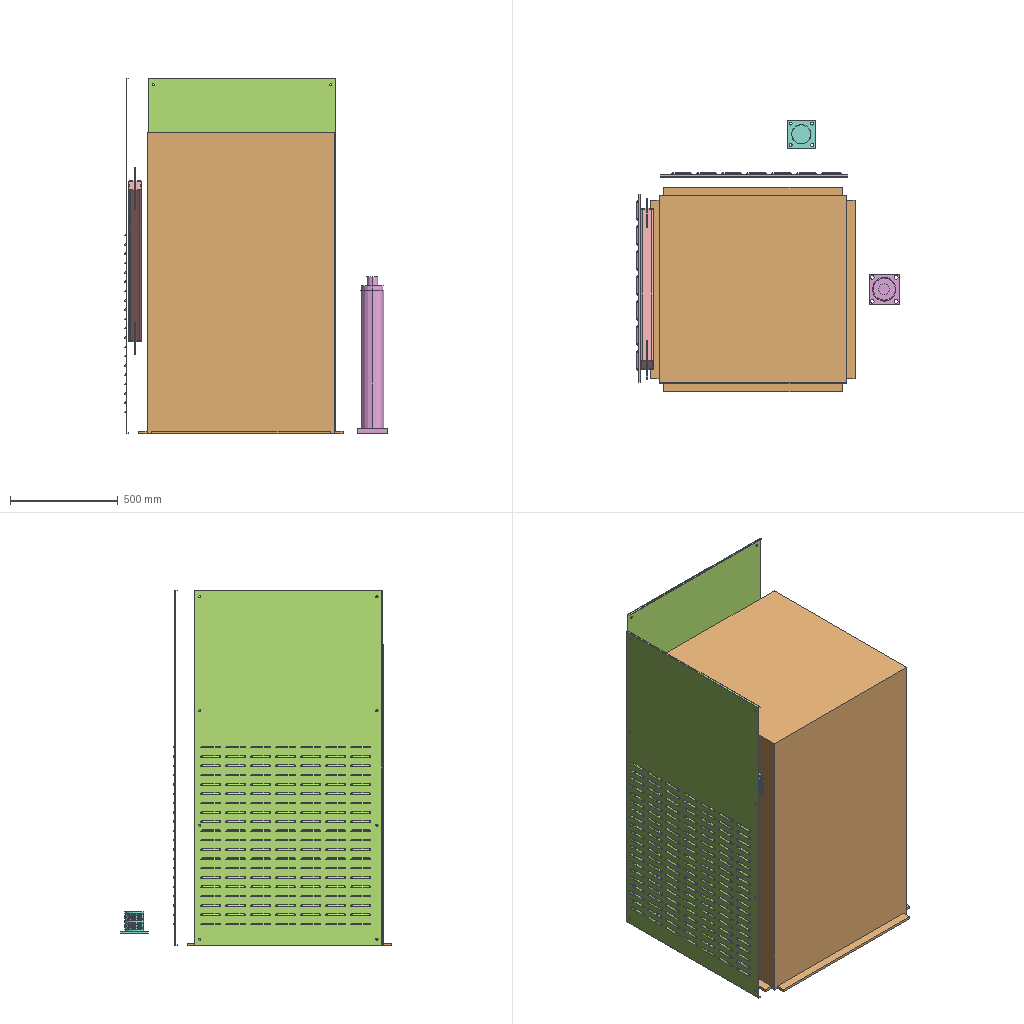Assembly | SolidWorks | 10 different items | 12 placed | box 1219 x 1260 x 1650 mm
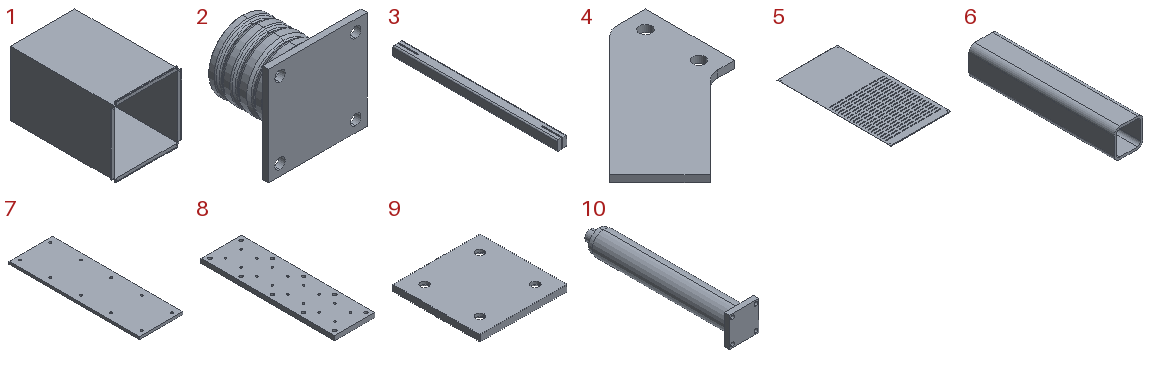Parts list (item | quantity | size | volume | features):
1 | x1 | 950 x 1400 x 950 mm | 61176455 mm3 | features CirPattern 1, Extrusion 1, ICE 1, RefAxis 1, Shell 1
2 | x1 | 130 x 100 x 130 mm | 689791 mm3 | features Chamfer 1, Extrusion 1, Fillet 1, ICE 1, RevCut 1
3 | x1 | 60 x 998 x 60 mm | 853297 mm3 | features ICE 3, Extrusion 1
4 | x2 | 181.644 x 197.856 x 8 mm | 132691 mm3 | features Extrusion 1
5 | x2 | 870 x 1650 x 17.75 mm | 2197633 mm3 | features ICE 5, Fillet 3, LPattern 2, Shell 2, CombineBodies 1, Extrusion 1
6 | x1 | 50 x 250 x 50 mm | 170265 mm3 | features Extrusion 1
7 | x1 | 100 x 300 x 6 mm | 178822 mm3 | features LPattern 2, Extrusion 1, HoleWzd 1
8 | x1 | 90 x 300 x 10 mm | 263935 mm3 | features LPattern 3, HoleWzd 2, Extrusion 1
9 | x1 | 55 x 55 x 4 mm | 11573 mm3 | features Chamfer 1, Extrusion 1, HoleWzd 1
10 | x1 | 140 x 729 x 140 mm | 6809578 mm3 | features ICE 1, Revolution 1
Mates (type | each side: item.copy, entity, surface, feature):
Coincident | 1.1 plane | assembly plane | 2 times
Parallel | 3.1 face plane Boss-Extrude1 | 4.1 face plane Boss-Extrude1
Coincident | 3.1 face plane Cut-Extrude1 | 4.1 face plane Boss-Extrude1
DistanceDim | 3.1 face plane Boss-Extrude1 | 4.1 edge
DistanceDim | 3.1 edge | 4.1 face plane Boss-Extrude1
Parallel | 3.1 face plane Cut-Extrude1 | 4.2 face plane Boss-Extrude1
Parallel | 3.1 face plane Boss-Extrude1 | 4.2 face plane Boss-Extrude1
DistanceDim | 3.1 face plane Boss-Extrude1 | 4.2 face plane Boss-Extrude1
DistanceDim | 3.1 edge | 4.2 face plane Boss-Extrude1
DistanceDim | 4.2 face plane Boss-Extrude1 | 3.1 face plane Cut-Extrude1
Coincident | 6.1 face plane Boss-Extrude1 | 7.1 face plane Boss-Extrude1
Parallel | 6.1 face plane Boss-Extrude1 | 7.1 face plane Boss-Extrude1
DistanceDim | 7.1 face plane Boss-Extrude1 | 6.1 face plane Boss-Extrude1
Coincident | 7.1 face plane Boss-Extrude1 | 8.1 face plane Boss-Extrude1
Concentric | 7.1 face cylinder LPattern2 | 8.1 face cylinder LPattern2
Coincident | 8.1 face plane Boss-Extrude1 | 9.1 face plane Boss-Extrude1
Concentric | 8.1 face cylinder LPattern3 | 9.1 face cylinder Ø1.0 (5.1) Diameter Hole1
Concentric | 8.1 face cylinder M5 Tapped Hole1 | assembly face